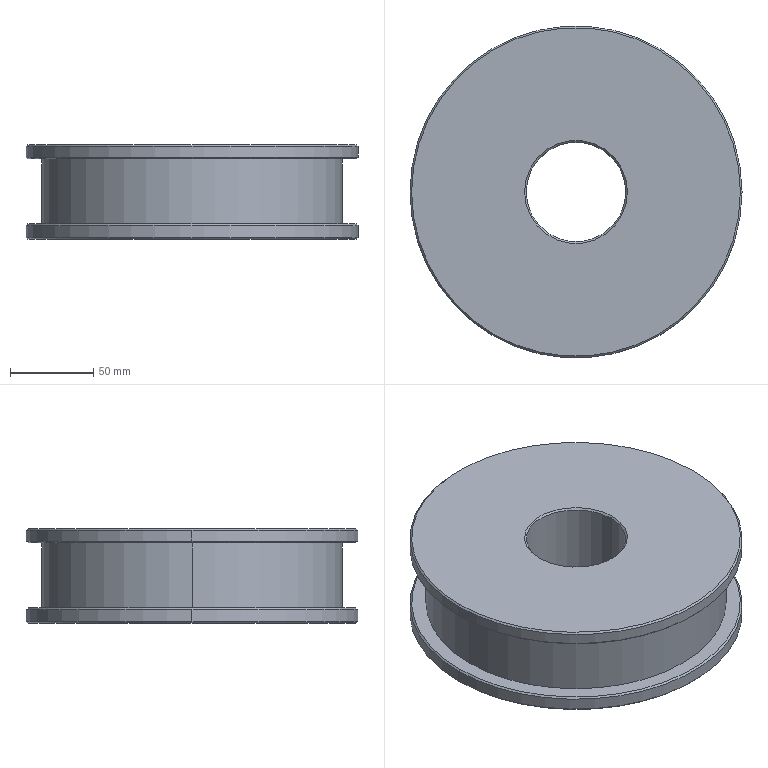Part | Creo | features DATUM PLANE 3, CHAMFER 1, COORDINATE SYSTEM 1, CURVE 1, CUT 1, PROTRUSION 1 | 1 solid | 24 faces | box 200 x 200 x 57 mm | volume 1403837 mm3 | cone 12 | cylinder 8 | plane 4 | commonest cylinder face diameters 200 x4 60 x2 180.852 x2
STEP:
#1=CARTESIAN_POINT('',(0.,0.,0.));
#2=DIRECTION('',(0.,0.,1.));
#3=DIRECTION('',(1.,0.,0.));
#4=AXIS2_PLACEMENT_3D('',#1,#2,#3);
#5=CARTESIAN_POINT('',(99.,0.,0.));
#6=VERTEX_POINT('',#5);
#7=CARTESIAN_POINT('',(-99.,0.,0.));
#8=VERTEX_POINT('',#7);
#9=CARTESIAN_POINT('',(0.,0.,0.));
#10=DIRECTION('',(0.,0.,-1.));
#11=DIRECTION('',(1.,0.,0.));
#12=AXIS2_PLACEMENT_3D('',#9,#10,#11);
#13=CIRCLE('',#12,99.);
#14=EDGE_CURVE('',#6,#8,#13,.T.);
#15=ORIENTED_EDGE('',*,*,#14,.F.);
#16=CARTESIAN_POINT('',(0.,0.,0.));
#17=DIRECTION('',(0.,0.,-1.));
#18=DIRECTION('',(-1.,0.,0.));
#19=AXIS2_PLACEMENT_3D('',#16,#17,#18);
#20=CIRCLE('',#19,99.);
#21=EDGE_CURVE('',#8,#6,#20,.T.);
#22=ORIENTED_EDGE('',*,*,#21,.F.);
#23=EDGE_LOOP('',(#15,#22));
#24=FACE_OUTER_BOUND('',#23,.F.);
#25=CARTESIAN_POINT('',(-31.,0.,0.));
#26=VERTEX_POINT('',#25);
#27=CARTESIAN_POINT('',(31.,0.,0.));
#28=VERTEX_POINT('',#27);
#29=CARTESIAN_POINT('',(0.,0.,0.));
#30=DIRECTION('',(0.,0.,1.));
#31=DIRECTION('',(-1.,0.,0.));
#32=AXIS2_PLACEMENT_3D('',#29,#30,#31);
#33=CIRCLE('',#32,31.);
#34=EDGE_CURVE('',#26,#28,#33,.T.);
#35=ORIENTED_EDGE('',*,*,#34,.F.);
#36=CARTESIAN_POINT('',(0.,0.,0.));
#37=DIRECTION('',(0.,0.,1.));
#38=DIRECTION('',(1.,0.,0.));
#39=AXIS2_PLACEMENT_3D('',#36,#37,#38);
#40=CIRCLE('',#39,31.);
#41=EDGE_CURVE('',#28,#26,#40,.T.);
#42=ORIENTED_EDGE('',*,*,#41,.F.);
#43=EDGE_LOOP('',(#35,#42));
#44=FACE_BOUND('',#43,.F.);
#45=CARTESIAN_POINT('',(0.,0.,0.));
#46=DIRECTION('',(0.,0.,1.));
#47=DIRECTION('',(1.,0.,0.));
#48=AXIS2_PLACEMENT_3D('',#45,#46,#47);
#49=PLANE('',#48);
#50=ADVANCED_FACE('',(#24,#44),#49,.F.);
#51=ORIENTED_EDGE('',*,*,#14,.T.);
#52=CARTESIAN_POINT('',(-100.,0.,1.));
#53=VERTEX_POINT('',#52);
#54=CARTESIAN_POINT('',(-99.,-0.000000016,0.));
#55=DIRECTION('',(-0.7071,0.000000003,0.7071));
#56=VECTOR('',#55,1.414);
#57=LINE('',#54,#56);
#58=EDGE_CURVE('',#8,#53,#57,.T.);
#59=ORIENTED_EDGE('',*,*,#58,.T.);
#60=CARTESIAN_POINT('',(100.,0.,1.));
#61=VERTEX_POINT('',#60);
#62=CARTESIAN_POINT('',(0.,0.,1.));
#63=DIRECTION('',(0.,0.,-1.));
#64=DIRECTION('',(1.,0.,0.));
#65=AXIS2_PLACEMENT_3D('',#62,#63,#64);
#66=CIRCLE('',#65,100.);
#67=EDGE_CURVE('',#61,#53,#66,.T.);
#68=ORIENTED_EDGE('',*,*,#67,.F.);
#69=CARTESIAN_POINT('',(99.,0.000000016,0.));
#70=DIRECTION('',(0.7071,-0.000000003,0.7071));
#71=VECTOR('',#70,1.414);
#72=LINE('',#69,#71);
#73=EDGE_CURVE('',#6,#61,#72,.T.);
#74=ORIENTED_EDGE('',*,*,#73,.F.);
#75=EDGE_LOOP('',(#51,#59,#68,#74));
#76=FACE_OUTER_BOUND('',#75,.F.);
#77=CARTESIAN_POINT('',(0.,0.,0.5));
#78=DIRECTION('',(0.,0.,1.));
#79=DIRECTION('',(0.,-1.,0.));
#80=AXIS2_PLACEMENT_3D('',#77,#78,#79);
#81=CONICAL_SURFACE('',#80,99.5,45.);
#82=ADVANCED_FACE('',(#76),#81,.T.);
#83=ORIENTED_EDGE('',*,*,#21,.T.);
#84=ORIENTED_EDGE('',*,*,#73,.T.);
#85=CARTESIAN_POINT('',(0.,0.,1.));
#86=DIRECTION('',(0.,0.,-1.));
#87=DIRECTION('',(-1.,0.,0.));
#88=AXIS2_PLACEMENT_3D('',#85,#86,#87);
#89=CIRCLE('',#88,100.);
#90=EDGE_CURVE('',#53,#61,#89,.T.);
#91=ORIENTED_EDGE('',*,*,#90,.F.);
#92=ORIENTED_EDGE('',*,*,#58,.F.);
#93=EDGE_LOOP('',(#83,#84,#91,#92));
#94=FACE_OUTER_BOUND('',#93,.F.);
#95=CARTESIAN_POINT('',(0.,0.,0.5));
#96=DIRECTION('',(0.,0.,1.));
#97=DIRECTION('',(0.,-1.,0.));
#98=AXIS2_PLACEMENT_3D('',#95,#96,#97);
#99=CONICAL_SURFACE('',#98,99.5,45.);
#100=ADVANCED_FACE('',(#94),#99,.T.);
#101=CARTESIAN_POINT('',(-100.,0.,8.269));
#102=VERTEX_POINT('',#101);
#103=CARTESIAN_POINT('',(100.,0.,8.269));
#104=VERTEX_POINT('',#103);
#105=CARTESIAN_POINT('',(0.,0.,8.269));
#106=DIRECTION('',(0.,0.,-1.));
#107=DIRECTION('',(-1.,0.,0.));
#108=AXIS2_PLACEMENT_3D('',#105,#106,#107);
#109=CIRCLE('',#108,100.);
#110=EDGE_CURVE('',#102,#104,#109,.T.);
#111=ORIENTED_EDGE('',*,*,#110,.F.);
#112=CARTESIAN_POINT('',(-100.,-0.000000012,1.));
#113=DIRECTION('',(0.,0.000000002,1.));
#114=VECTOR('',#113,7.269);
#115=LINE('',#112,#114);
#116=EDGE_CURVE('',#53,#102,#115,.T.);
#117=ORIENTED_EDGE('',*,*,#116,.F.);
#118=ORIENTED_EDGE('',*,*,#90,.T.);
#119=CARTESIAN_POINT('',(100.,0.000000012,1.));
#120=DIRECTION('',(0.,-0.000000002,1.));
#121=VECTOR('',#120,7.269);
#122=LINE('',#119,#121);
#123=EDGE_CURVE('',#61,#104,#122,.T.);
#124=ORIENTED_EDGE('',*,*,#123,.T.);
#125=EDGE_LOOP('',(#111,#117,#118,#124));
#126=FACE_OUTER_BOUND('',#125,.F.);
#127=CARTESIAN_POINT('',(0.,0.,0.));
#128=DIRECTION('',(0.,0.,1.));
#129=DIRECTION('',(1.,0.,0.));
#130=AXIS2_PLACEMENT_3D('',#127,#128,#129);
#131=CYLINDRICAL_SURFACE('',#130,100.);
#132=ADVANCED_FACE('',(#126),#131,.T.);
#133=CARTESIAN_POINT('',(100.,0.,49.424));
#134=VERTEX_POINT('',#133);
#135=CARTESIAN_POINT('',(-100.,0.,49.424));
#136=VERTEX_POINT('',#135);
#137=CARTESIAN_POINT('',(0.,0.,49.424));
#138=DIRECTION('',(0.,0.,1.));
#139=DIRECTION('',(1.,0.,0.));
#140=AXIS2_PLACEMENT_3D('',#137,#138,#139);
#141=CIRCLE('',#140,100.);
#142=EDGE_CURVE('',#134,#136,#141,.T.);
#143=ORIENTED_EDGE('',*,*,#142,.F.);
#144=CARTESIAN_POINT('',(100.,0.,56.));
#145=VERTEX_POINT('',#144);
#146=CARTESIAN_POINT('',(100.,-0.000000003,49.424));
#147=DIRECTION('',(0.,0.000000002,1.));
#148=VECTOR('',#147,6.576);
#149=LINE('',#146,#148);
#150=EDGE_CURVE('',#134,#145,#149,.T.);
#151=ORIENTED_EDGE('',*,*,#150,.T.);
#152=CARTESIAN_POINT('',(-100.,0.,56.));
#153=VERTEX_POINT('',#152);
#154=CARTESIAN_POINT('',(0.,0.,56.));
#155=DIRECTION('',(0.,0.,1.));
#156=DIRECTION('',(1.,0.,0.));
#157=AXIS2_PLACEMENT_3D('',#154,#155,#156);
#158=CIRCLE('',#157,100.);
#159=EDGE_CURVE('',#145,#153,#158,.T.);
#160=ORIENTED_EDGE('',*,*,#159,.T.);
#161=CARTESIAN_POINT('',(-100.,0.000000003,49.424));
#162=DIRECTION('',(0.,-0.000000002,1.));
#163=VECTOR('',#162,6.576);
#164=LINE('',#161,#163);
#165=EDGE_CURVE('',#136,#153,#164,.T.);
#166=ORIENTED_EDGE('',*,*,#165,.F.);
#167=EDGE_LOOP('',(#143,#151,#160,#166));
#168=FACE_OUTER_BOUND('',#167,.F.);
#169=CARTESIAN_POINT('',(0.,0.,0.));
#170=DIRECTION('',(0.,0.,1.));
#171=DIRECTION('',(1.,0.,0.));
#172=AXIS2_PLACEMENT_3D('',#169,#170,#171);
#173=CYLINDRICAL_SURFACE('',#172,100.);
#174=ADVANCED_FACE('',(#168),#173,.T.);
#175=ORIENTED_EDGE('',*,*,#110,.T.);
#176=CARTESIAN_POINT('',(99.,0.,9.269));
#177=VERTEX_POINT('',#176);
#178=CARTESIAN_POINT('',(100.,-0.000000003,8.269));
#179=DIRECTION('',(-0.7071,-0.000000001,0.7071));
#180=VECTOR('',#179,1.414);
#181=LINE('',#178,#180);
#182=EDGE_CURVE('',#104,#177,#181,.T.);
#183=ORIENTED_EDGE('',*,*,#182,.T.);
#184=CARTESIAN_POINT('',(-99.,0.,9.269));
#185=VERTEX_POINT('',#184);
#186=CARTESIAN_POINT('',(0.,0.,9.269));
#187=DIRECTION('',(0.,0.,-1.));
#188=DIRECTION('',(-1.,0.,0.));
#189=AXIS2_PLACEMENT_3D('',#186,#187,#188);
#190=CIRCLE('',#189,99.);
#191=EDGE_CURVE('',#185,#177,#190,.T.);
#192=ORIENTED_EDGE('',*,*,#191,.F.);
#193=CARTESIAN_POINT('',(-100.,0.000000003,8.269));
#194=DIRECTION('',(0.7071,0.000000001,0.7071));
#195=VECTOR('',#194,1.414);
#196=LINE('',#193,#195);
#197=EDGE_CURVE('',#102,#185,#196,.T.);
#198=ORIENTED_EDGE('',*,*,#197,.F.);
#199=EDGE_LOOP('',(#175,#183,#192,#198));
#200=FACE_OUTER_BOUND('',#199,.F.);
#201=CARTESIAN_POINT('',(0.,0.,8.769));
#202=DIRECTION('',(0.,0.,-1.));
#203=DIRECTION('',(0.,-1.,0.));
#204=AXIS2_PLACEMENT_3D('',#201,#202,#203);
#205=CONICAL_SURFACE('',#204,99.5,45.);
#206=ADVANCED_FACE('',(#200),#205,.T.);
#207=CARTESIAN_POINT('',(0.,0.,8.269));
#208=DIRECTION('',(0.,0.,-1.));
#209=DIRECTION('',(1.,0.,0.));
#210=AXIS2_PLACEMENT_3D('',#207,#208,#209);
#211=CIRCLE('',#210,100.);
#212=EDGE_CURVE('',#104,#102,#211,.T.);
#213=ORIENTED_EDGE('',*,*,#212,.T.);
#214=ORIENTED_EDGE('',*,*,#197,.T.);
#215=CARTESIAN_POINT('',(0.,0.,9.269));
#216=DIRECTION('',(0.,0.,-1.));
#217=DIRECTION('',(1.,0.,0.));
#218=AXIS2_PLACEMENT_3D('',#215,#216,#217);
#219=CIRCLE('',#218,99.);
#220=EDGE_CURVE('',#177,#185,#219,.T.);
#221=ORIENTED_EDGE('',*,*,#220,.F.);
#222=ORIENTED_EDGE('',*,*,#182,.F.);
#223=EDGE_LOOP('',(#213,#214,#221,#222));
#224=FACE_OUTER_BOUND('',#223,.F.);
#225=CARTESIAN_POINT('',(0.,0.,8.769));
#226=DIRECTION('',(0.,0.,-1.));
#227=DIRECTION('',(0.,-1.,0.));
#228=AXIS2_PLACEMENT_3D('',#225,#226,#227);
#229=CONICAL_SURFACE('',#228,99.5,45.);
#230=ADVANCED_FACE('',(#224),#229,.T.);
#231=ORIENTED_EDGE('',*,*,#212,.F.);
#232=ORIENTED_EDGE('',*,*,#123,.F.);
#233=ORIENTED_EDGE('',*,*,#67,.T.);
#234=ORIENTED_EDGE('',*,*,#116,.T.);
#235=EDGE_LOOP('',(#231,#232,#233,#234));
#236=FACE_OUTER_BOUND('',#235,.F.);
#237=CARTESIAN_POINT('',(0.,0.,0.));
#238=DIRECTION('',(0.,0.,1.));
#239=DIRECTION('',(1.,0.,0.));
#240=AXIS2_PLACEMENT_3D('',#237,#238,#239);
#241=CYLINDRICAL_SURFACE('',#240,100.);
#242=ADVANCED_FACE('',(#236),#241,.T.);
#243=CARTESIAN_POINT('',(0.,0.,49.424));
#244=DIRECTION('',(0.,0.,1.));
#245=DIRECTION('',(-1.,0.,0.));
#246=AXIS2_PLACEMENT_3D('',#243,#244,#245);
#247=CIRCLE('',#246,100.);
#248=EDGE_CURVE('',#136,#134,#247,.T.);
#249=ORIENTED_EDGE('',*,*,#248,.F.);
#250=ORIENTED_EDGE('',*,*,#165,.T.);
#251=CARTESIAN_POINT('',(0.,0.,56.));
#252=DIRECTION('',(0.,0.,1.));
#253=DIRECTION('',(-1.,0.,0.));
#254=AXIS2_PLACEMENT_3D('',#251,#252,#253);
#255=CIRCLE('',#254,100.);
#256=EDGE_CURVE('',#153,#145,#255,.T.);
#257=ORIENTED_EDGE('',*,*,#256,.T.);
#258=ORIENTED_EDGE('',*,*,#150,.F.);
#259=EDGE_LOOP('',(#249,#250,#257,#258));
#260=FACE_OUTER_BOUND('',#259,.F.);
#261=CARTESIAN_POINT('',(0.,0.,0.));
#262=DIRECTION('',(0.,0.,1.));
#263=DIRECTION('',(1.,0.,0.));
#264=AXIS2_PLACEMENT_3D('',#261,#262,#263);
#265=CYLINDRICAL_SURFACE('',#264,100.);
#266=ADVANCED_FACE('',(#260),#265,.T.);
#267=ORIENTED_EDGE('',*,*,#248,.T.);
#268=CARTESIAN_POINT('',(99.,0.,48.424));
#269=VERTEX_POINT('',#268);
#270=CARTESIAN_POINT('',(100.,-0.000000003,49.424));
#271=DIRECTION('',(-0.7071,-0.000000001,-0.7071));
#272=VECTOR('',#271,1.414);
#273=LINE('',#270,#272);
#274=EDGE_CURVE('',#134,#269,#273,.T.);
#275=ORIENTED_EDGE('',*,*,#274,.T.);
#276=CARTESIAN_POINT('',(-99.,0.,48.424));
#277=VERTEX_POINT('',#276);
#278=CARTESIAN_POINT('',(0.,0.,48.424));
#279=DIRECTION('',(0.,0.,1.));
#280=DIRECTION('',(-1.,0.,0.));
#281=AXIS2_PLACEMENT_3D('',#278,#279,#280);
#282=CIRCLE('',#281,99.);
#283=EDGE_CURVE('',#277,#269,#282,.T.);
#284=ORIENTED_EDGE('',*,*,#283,.F.);
#285=CARTESIAN_POINT('',(-100.,0.000000003,49.424));
#286=DIRECTION('',(0.7071,0.000000001,-0.7071));
#287=VECTOR('',#286,1.414);
#288=LINE('',#285,#287);
#289=EDGE_CURVE('',#136,#277,#288,.T.);
#290=ORIENTED_EDGE('',*,*,#289,.F.);
#291=EDGE_LOOP('',(#267,#275,#284,#290));
#292=FACE_OUTER_BOUND('',#291,.F.);
#293=CARTESIAN_POINT('',(0.,0.,48.924));
#294=DIRECTION('',(0.,0.,1.));
#295=DIRECTION('',(0.,-1.,0.));
#296=AXIS2_PLACEMENT_3D('',#293,#294,#295);
#297=CONICAL_SURFACE('',#296,99.5,45.);
#298=ADVANCED_FACE('',(#292),#297,.T.);
#299=ORIENTED_EDGE('',*,*,#142,.T.);
#300=ORIENTED_EDGE('',*,*,#289,.T.);
#301=CARTESIAN_POINT('',(0.,0.,48.424));
#302=DIRECTION('',(0.,0.,1.));
#303=DIRECTION('',(1.,0.,0.));
#304=AXIS2_PLACEMENT_3D('',#301,#302,#303);
#305=CIRCLE('',#304,99.);
#306=EDGE_CURVE('',#269,#277,#305,.T.);
#307=ORIENTED_EDGE('',*,*,#306,.F.);
#308=ORIENTED_EDGE('',*,*,#274,.F.);
#309=EDGE_LOOP('',(#299,#300,#307,#308));
#310=FACE_OUTER_BOUND('',#309,.F.);
#311=CARTESIAN_POINT('',(0.,0.,48.924));
#312=DIRECTION('',(0.,0.,1.));
#313=DIRECTION('',(0.,-1.,0.));
#314=AXIS2_PLACEMENT_3D('',#311,#312,#313);
#315=CONICAL_SURFACE('',#314,99.5,45.);
#316=ADVANCED_FACE('',(#310),#315,.T.);
#317=ORIENTED_EDGE('',*,*,#283,.T.);
#318=ORIENTED_EDGE('',*,*,#306,.T.);
#319=EDGE_LOOP('',(#317,#318));
#320=FACE_OUTER_BOUND('',#319,.F.);
#321=CARTESIAN_POINT('',(-90.426,0.,48.424));
#322=VERTEX_POINT('',#321);
#323=CARTESIAN_POINT('',(90.426,0.,48.424));
#324=VERTEX_POINT('',#323);
#325=CARTESIAN_POINT('',(0.,0.,48.424));
#326=DIRECTION('',(0.,0.,1.));
#327=DIRECTION('',(-1.,0.,0.));
#328=AXIS2_PLACEMENT_3D('',#325,#326,#327);
#329=CIRCLE('',#328,90.426);
#330=EDGE_CURVE('',#322,#324,#329,.T.);
#331=ORIENTED_EDGE('',*,*,#330,.F.);
#332=CARTESIAN_POINT('',(0.,0.,48.424));
#333=DIRECTION('',(0.,0.,1.));
#334=DIRECTION('',(1.,0.,0.));
#335=AXIS2_PLACEMENT_3D('',#332,#333,#334);
#336=CIRCLE('',#335,90.426);
#337=EDGE_CURVE('',#324,#322,#336,.T.);
#338=ORIENTED_EDGE('',*,*,#337,.F.);
#339=EDGE_LOOP('',(#331,#338));
#340=FACE_BOUND('',#339,.F.);
#341=CARTESIAN_POINT('',(0.,0.,48.424));
#342=DIRECTION('',(0.,0.,1.));
#343=DIRECTION('',(1.,0.,0.));
#344=AXIS2_PLACEMENT_3D('',#341,#342,#343);
#345=PLANE('',#344);
#346=ADVANCED_FACE('',(#320,#340),#345,.F.);
#347=CARTESIAN_POINT('',(-90.426,0.,9.269));
#348=VERTEX_POINT('',#347);
#349=CARTESIAN_POINT('',(-90.426,0.,9.269));
#350=DIRECTION('',(0.,0.,1.));
#351=VECTOR('',#350,39.155);
#352=LINE('',#349,#351);
#353=EDGE_CURVE('',#348,#322,#352,.T.);
#354=ORIENTED_EDGE('',*,*,#353,.T.);
#355=ORIENTED_EDGE('',*,*,#330,.T.);
#356=CARTESIAN_POINT('',(90.426,0.,9.269));
#357=VERTEX_POINT('',#356);
#358=CARTESIAN_POINT('',(90.426,0.,9.269));
#359=DIRECTION('',(0.,0.,1.));
#360=VECTOR('',#359,39.155);
#361=LINE('',#358,#360);
#362=EDGE_CURVE('',#357,#324,#361,.T.);
#363=ORIENTED_EDGE('',*,*,#362,.F.);
#364=CARTESIAN_POINT('',(0.,0.,9.269));
#365=DIRECTION('',(0.,0.,1.));
#366=DIRECTION('',(-1.,0.,0.));
#367=AXIS2_PLACEMENT_3D('',#364,#365,#366);
#368=CIRCLE('',#367,90.426);
#369=EDGE_CURVE('',#348,#357,#368,.T.);
#370=ORIENTED_EDGE('',*,*,#369,.F.);
#371=EDGE_LOOP('',(#354,#355,#363,#370));
#372=FACE_OUTER_BOUND('',#371,.F.);
#373=CARTESIAN_POINT('',(0.,0.,56.));
#374=DIRECTION('',(0.,0.,1.));
#375=DIRECTION('',(1.,0.,0.));
#376=AXIS2_PLACEMENT_3D('',#373,#374,#375);
#377=CYLINDRICAL_SURFACE('',#376,90.426);
#378=ADVANCED_FACE('',(#372),#377,.T.);
#379=ORIENTED_EDGE('',*,*,#362,.T.);
#380=ORIENTED_EDGE('',*,*,#337,.T.);
#381=ORIENTED_EDGE('',*,*,#353,.F.);
#382=CARTESIAN_POINT('',(0.,0.,9.269));
#383=DIRECTION('',(0.,0.,1.));
#384=DIRECTION('',(1.,0.,0.));
#385=AXIS2_PLACEMENT_3D('',#382,#383,#384);
#386=CIRCLE('',#385,90.426);
#387=EDGE_CURVE('',#357,#348,#386,.T.);
#388=ORIENTED_EDGE('',*,*,#387,.F.);
#389=EDGE_LOOP('',(#379,#380,#381,#388));
#390=FACE_OUTER_BOUND('',#389,.F.);
#391=CARTESIAN_POINT('',(0.,0.,56.));
#392=DIRECTION('',(0.,0.,1.));
#393=DIRECTION('',(-1.,0.,0.));
#394=AXIS2_PLACEMENT_3D('',#391,#392,#393);
#395=CYLINDRICAL_SURFACE('',#394,90.426);
#396=ADVANCED_FACE('',(#390),#395,.T.);
#397=ORIENTED_EDGE('',*,*,#220,.T.);
#398=ORIENTED_EDGE('',*,*,#191,.T.);
#399=EDGE_LOOP('',(#397,#398));
#400=FACE_OUTER_BOUND('',#399,.F.);
#401=ORIENTED_EDGE('',*,*,#387,.T.);
#402=ORIENTED_EDGE('',*,*,#369,.T.);
#403=EDGE_LOOP('',(#401,#402));
#404=FACE_BOUND('',#403,.F.);
#405=CARTESIAN_POINT('',(0.,0.,9.269));
#406=DIRECTION('',(0.,0.,1.));
#407=DIRECTION('',(1.,0.,0.));
#408=AXIS2_PLACEMENT_3D('',#405,#406,#407);
#409=PLANE('',#408);
#410=ADVANCED_FACE('',(#400,#404),#409,.T.);
#411=CARTESIAN_POINT('',(-99.,0.,57.));
#412=VERTEX_POINT('',#411);
#413=CARTESIAN_POINT('',(99.,0.,57.));
#414=VERTEX_POINT('',#413);
#415=CARTESIAN_POINT('',(0.,0.,57.));
#416=DIRECTION('',(0.,0.,1.));
#417=DIRECTION('',(-1.,0.,0.));
#418=AXIS2_PLACEMENT_3D('',#415,#416,#417);
#419=CIRCLE('',#418,99.);
#420=EDGE_CURVE('',#412,#414,#419,.T.);
#421=ORIENTED_EDGE('',*,*,#420,.T.);
#422=CARTESIAN_POINT('',(99.,0.000000016,57.));
#423=DIRECTION('',(0.7071,-0.000000003,-0.7071));
#424=VECTOR('',#423,1.414);
#425=LINE('',#422,#424);
#426=EDGE_CURVE('',#414,#145,#425,.T.);
#427=ORIENTED_EDGE('',*,*,#426,.T.);
#428=ORIENTED_EDGE('',*,*,#256,.F.);
#429=CARTESIAN_POINT('',(-99.,-0.000000016,57.));
#430=DIRECTION('',(-0.7071,0.000000003,-0.7071));
#431=VECTOR('',#430,1.414);
#432=LINE('',#429,#431);
#433=EDGE_CURVE('',#412,#153,#432,.T.);
#434=ORIENTED_EDGE('',*,*,#433,.F.);
#435=EDGE_LOOP('',(#421,#427,#428,#434));
#436=FACE_OUTER_BOUND('',#435,.F.);
#437=CARTESIAN_POINT('',(0.,0.,56.5));
#438=DIRECTION('',(0.,0.,-1.));
#439=DIRECTION('',(0.,-1.,0.));
#440=AXIS2_PLACEMENT_3D('',#437,#438,#439);
#441=CONICAL_SURFACE('',#440,99.5,45.);
#442=ADVANCED_FACE('',(#436),#441,.T.);
#443=ORIENTED_EDGE('',*,*,#420,.F.);
#444=CARTESIAN_POINT('',(0.,0.,57.));
#445=DIRECTION('',(0.,0.,1.));
#446=DIRECTION('',(1.,0.,0.));
#447=AXIS2_PLACEMENT_3D('',#444,#445,#446);
#448=CIRCLE('',#447,99.);
#449=EDGE_CURVE('',#414,#412,#448,.T.);
#450=ORIENTED_EDGE('',*,*,#449,.F.);
#451=EDGE_LOOP('',(#443,#450));
#452=FACE_OUTER_BOUND('',#451,.F.);
#453=CARTESIAN_POINT('',(31.,0.,57.));
#454=VERTEX_POINT('',#453);
#455=CARTESIAN_POINT('',(-31.,0.,57.));
#456=VERTEX_POINT('',#455);
#457=CARTESIAN_POINT('',(0.,0.,57.));
#458=DIRECTION('',(0.,0.,-1.));
#459=DIRECTION('',(1.,0.,0.));
#460=AXIS2_PLACEMENT_3D('',#457,#458,#459);
#461=CIRCLE('',#460,31.);
#462=EDGE_CURVE('',#454,#456,#461,.T.);
#463=ORIENTED_EDGE('',*,*,#462,.F.);
#464=CARTESIAN_POINT('',(0.,0.,57.));
#465=DIRECTION('',(0.,0.,-1.));
#466=DIRECTION('',(-1.,0.,0.));
#467=AXIS2_PLACEMENT_3D('',#464,#465,#466);
#468=CIRCLE('',#467,31.);
#469=EDGE_CURVE('',#456,#454,#468,.T.);
#470=ORIENTED_EDGE('',*,*,#469,.F.);
#471=EDGE_LOOP('',(#463,#470));
#472=FACE_BOUND('',#471,.F.);
#473=CARTESIAN_POINT('',(0.,0.,57.));
#474=DIRECTION('',(0.,0.,1.));
#475=DIRECTION('',(1.,0.,0.));
#476=AXIS2_PLACEMENT_3D('',#473,#474,#475);
#477=PLANE('',#476);
#478=ADVANCED_FACE('',(#452,#472),#477,.T.);
#479=ORIENTED_EDGE('',*,*,#449,.T.);
#480=ORIENTED_EDGE('',*,*,#433,.T.);
#481=ORIENTED_EDGE('',*,*,#159,.F.);
#482=ORIENTED_EDGE('',*,*,#426,.F.);
#483=EDGE_LOOP('',(#479,#480,#481,#482));
#484=FACE_OUTER_BOUND('',#483,.F.);
#485=CARTESIAN_POINT('',(0.,0.,56.5));
#486=DIRECTION('',(0.,0.,-1.));
#487=DIRECTION('',(0.,-1.,0.));
#488=AXIS2_PLACEMENT_3D('',#485,#486,#487);
#489=CONICAL_SURFACE('',#488,99.5,45.);
#490=ADVANCED_FACE('',(#484),#489,.T.);
#491=ORIENTED_EDGE('',*,*,#462,.T.);
#492=CARTESIAN_POINT('',(-30.,0.,56.));
#493=VERTEX_POINT('',#492);
#494=CARTESIAN_POINT('',(-31.,-0.000000018,57.));
#495=DIRECTION('',(0.7071,0.000000004,-0.7071));
#496=VECTOR('',#495,1.414);
#497=LINE('',#494,#496);
#498=EDGE_CURVE('',#456,#493,#497,.T.);
#499=ORIENTED_EDGE('',*,*,#498,.T.);
#500=CARTESIAN_POINT('',(30.,0.,56.));
#501=VERTEX_POINT('',#500);
#502=CARTESIAN_POINT('',(0.,0.,56.));
#503=DIRECTION('',(0.,0.,-1.));
#504=DIRECTION('',(1.,0.,0.));
#505=AXIS2_PLACEMENT_3D('',#502,#503,#504);
#506=CIRCLE('',#505,30.);
#507=EDGE_CURVE('',#501,#493,#506,.T.);
#508=ORIENTED_EDGE('',*,*,#507,.F.);
#509=CARTESIAN_POINT('',(31.,0.000000018,57.));
#510=DIRECTION('',(-0.7071,-0.000000004,-0.7071));
#511=VECTOR('',#510,1.414);
#512=LINE('',#509,#511);
#513=EDGE_CURVE('',#454,#501,#512,.T.);
#514=ORIENTED_EDGE('',*,*,#513,.F.);
#515=EDGE_LOOP('',(#491,#499,#508,#514));
#516=FACE_OUTER_BOUND('',#515,.F.);
#517=CARTESIAN_POINT('',(0.,0.,56.5));
#518=DIRECTION('',(0.,0.,1.));
#519=DIRECTION('',(0.,-1.,0.));
#520=AXIS2_PLACEMENT_3D('',#517,#518,#519);
#521=CONICAL_SURFACE('',#520,30.5,45.);
#522=ADVANCED_FACE('',(#516),#521,.F.);
#523=ORIENTED_EDGE('',*,*,#469,.T.);
#524=ORIENTED_EDGE('',*,*,#513,.T.);
#525=CARTESIAN_POINT('',(0.,0.,56.));
#526=DIRECTION('',(0.,0.,-1.));
#527=DIRECTION('',(-1.,0.,0.));
#528=AXIS2_PLACEMENT_3D('',#525,#526,#527);
#529=CIRCLE('',#528,30.);
#530=EDGE_CURVE('',#493,#501,#529,.T.);
#531=ORIENTED_EDGE('',*,*,#530,.F.);
#532=ORIENTED_EDGE('',*,*,#498,.F.);
#533=EDGE_LOOP('',(#523,#524,#531,#532));
#534=FACE_OUTER_BOUND('',#533,.F.);
#535=CARTESIAN_POINT('',(0.,0.,56.5));
#536=DIRECTION('',(0.,0.,1.));
#537=DIRECTION('',(0.,-1.,0.));
#538=AXIS2_PLACEMENT_3D('',#535,#536,#537);
#539=CONICAL_SURFACE('',#538,30.5,45.);
#540=ADVANCED_FACE('',(#534),#539,.F.);
#541=CARTESIAN_POINT('',(30.,0.,1.));
#542=VERTEX_POINT('',#541);
#543=CARTESIAN_POINT('',(-30.,0.,1.));
#544=VERTEX_POINT('',#543);
#545=CARTESIAN_POINT('',(0.,0.,1.));
#546=DIRECTION('',(0.,0.,1.));
#547=DIRECTION('',(1.,0.,0.));
#548=AXIS2_PLACEMENT_3D('',#545,#546,#547);
#549=CIRCLE('',#548,30.);
#550=EDGE_CURVE('',#542,#544,#549,.T.);
#551=ORIENTED_EDGE('',*,*,#550,.T.);
#552=CARTESIAN_POINT('',(-30.,-0.000000013,1.));
#553=DIRECTION('',(0.,0.,1.));
#554=VECTOR('',#553,55.);
#555=LINE('',#552,#554);
#556=EDGE_CURVE('',#544,#493,#555,.T.);
#557=ORIENTED_EDGE('',*,*,#556,.T.);
#558=ORIENTED_EDGE('',*,*,#530,.T.);
#559=CARTESIAN_POINT('',(30.,0.000000013,1.));
#560=DIRECTION('',(0.,0.,1.));
#561=VECTOR('',#560,55.);
#562=LINE('',#559,#561);
#563=EDGE_CURVE('',#542,#501,#562,.T.);
#564=ORIENTED_EDGE('',*,*,#563,.F.);
#565=EDGE_LOOP('',(#551,#557,#558,#564));
#566=FACE_OUTER_BOUND('',#565,.F.);
#567=CARTESIAN_POINT('',(0.,0.,0.));
#568=DIRECTION('',(0.,0.,1.));
#569=DIRECTION('',(1.,0.,0.));
#570=AXIS2_PLACEMENT_3D('',#567,#568,#569);
#571=CYLINDRICAL_SURFACE('',#570,30.);
#572=ADVANCED_FACE('',(#566),#571,.F.);
#573=ORIENTED_EDGE('',*,*,#41,.T.);
#574=CARTESIAN_POINT('',(-31.,-0.000000018,0.000000005));
#575=DIRECTION('',(0.7071,0.000000004,0.7071));
#576=VECTOR('',#575,1.414);
#577=LINE('',#574,#576);
#578=EDGE_CURVE('',#26,#544,#577,.T.);
#579=ORIENTED_EDGE('',*,*,#578,.T.);
#580=ORIENTED_EDGE('',*,*,#550,.F.);
#581=CARTESIAN_POINT('',(31.,0.000000018,0.000000005));
#582=DIRECTION('',(-0.7071,-0.000000004,0.7071));
#583=VECTOR('',#582,1.414);
#584=LINE('',#581,#583);
#585=EDGE_CURVE('',#28,#542,#584,.T.);
#586=ORIENTED_EDGE('',*,*,#585,.F.);
#587=EDGE_LOOP('',(#573,#579,#580,#586));
#588=FACE_OUTER_BOUND('',#587,.F.);
#589=CARTESIAN_POINT('',(0.,0.,0.5));
#590=DIRECTION('',(0.,0.,-1.));
#591=DIRECTION('',(0.,-1.,0.));
#592=AXIS2_PLACEMENT_3D('',#589,#590,#591);
#593=CONICAL_SURFACE('',#592,30.5,45.);
#594=ADVANCED_FACE('',(#588),#593,.F.);
#595=ORIENTED_EDGE('',*,*,#34,.T.);
#596=ORIENTED_EDGE('',*,*,#585,.T.);
#597=CARTESIAN_POINT('',(0.,0.,1.));
#598=DIRECTION('',(0.,0.,1.));
#599=DIRECTION('',(-1.,0.,0.));
#600=AXIS2_PLACEMENT_3D('',#597,#598,#599);
#601=CIRCLE('',#600,30.);
#602=EDGE_CURVE('',#544,#542,#601,.T.);
#603=ORIENTED_EDGE('',*,*,#602,.F.);
#604=ORIENTED_EDGE('',*,*,#578,.F.);
#605=EDGE_LOOP('',(#595,#596,#603,#604));
#606=FACE_OUTER_BOUND('',#605,.F.);
#607=CARTESIAN_POINT('',(0.,0.,0.5));
#608=DIRECTION('',(0.,0.,-1.));
#609=DIRECTION('',(0.,-1.,0.));
#610=AXIS2_PLACEMENT_3D('',#607,#608,#609);
#611=CONICAL_SURFACE('',#610,30.5,45.);
#612=ADVANCED_FACE('',(#606),#611,.F.);
#613=ORIENTED_EDGE('',*,*,#602,.T.);
#614=ORIENTED_EDGE('',*,*,#563,.T.);
#615=ORIENTED_EDGE('',*,*,#507,.T.);
#616=ORIENTED_EDGE('',*,*,#556,.F.);
#617=EDGE_LOOP('',(#613,#614,#615,#616));
#618=FACE_OUTER_BOUND('',#617,.F.);
#619=CARTESIAN_POINT('',(0.,0.,0.));
#620=DIRECTION('',(0.,0.,1.));
#621=DIRECTION('',(1.,0.,0.));
#622=AXIS2_PLACEMENT_3D('',#619,#620,#621);
#623=CYLINDRICAL_SURFACE('',#622,30.);
#624=ADVANCED_FACE('',(#618),#623,.F.);
#625=CLOSED_SHELL('',(#50,#82,#100,#132,#174,#206,#230,#242,#266,#298,#316,#346,#378,#396,#410,#442,#478,#490,#522,#540,#572,#594,#612,#624));
#626=MANIFOLD_SOLID_BREP('',#625);
#627=(LENGTH_UNIT()NAMED_UNIT(*)SI_UNIT(.MILLI.,.METRE.));
#628=UNCERTAINTY_MEASURE_WITH_UNIT(LENGTH_MEASURE(0.02886),#627,'','');
#629=(NAMED_UNIT(*)PLANE_ANGLE_UNIT()SI_UNIT($,.RADIAN.));
#630=PLANE_ANGLE_MEASURE_WITH_UNIT(PLANE_ANGLE_MEASURE(0.01745),#629);
#631=(CONVERSION_BASED_UNIT('DEGREE',#630)NAMED_UNIT(*)PLANE_ANGLE_UNIT());
#632=(NAMED_UNIT(*)SI_UNIT($,.STERADIAN.)SOLID_ANGLE_UNIT());
#633=(GEOMETRIC_REPRESENTATION_CONTEXT(3)GLOBAL_UNCERTAINTY_ASSIGNED_CONTEXT((#628))GLOBAL_UNIT_ASSIGNED_CONTEXT((#627,#631,#632))REPRESENTATION_CONTEXT('',''));
#634=ADVANCED_BREP_SHAPE_REPRESENTATION('',(#4,#626),#633);